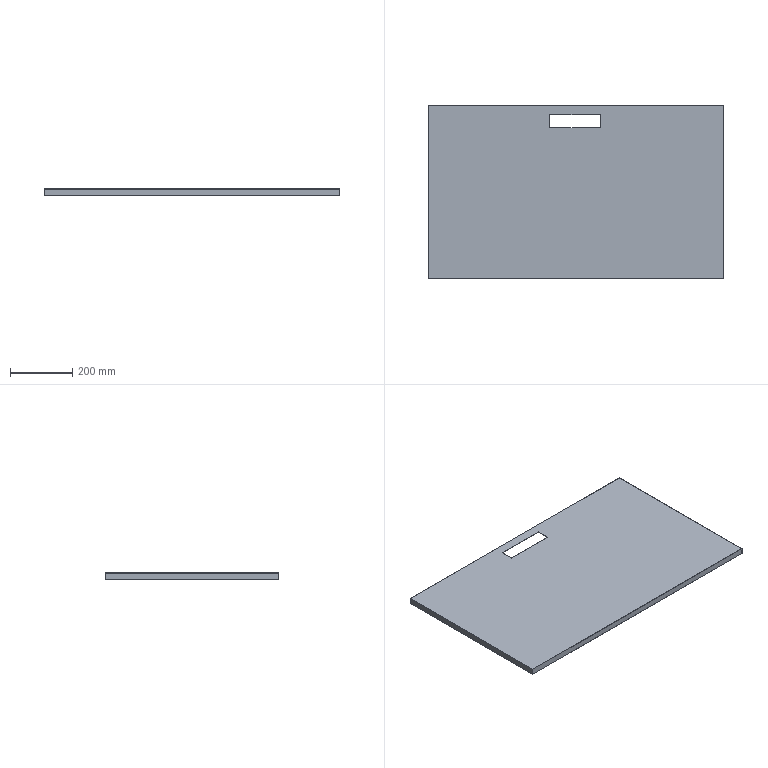Part | STEP file | PN_0019 | 1 solid | 15 faces | box 953 x 560 x 20 mm | volume 584212 mm3 | plane 15
STEP:
#1=CARTESIAN_POINT('',(0.,0.,0.));
#2=DIRECTION('',(0.,0.,1.));
#3=DIRECTION('',(1.,0.,0.));
#4=AXIS2_PLACEMENT_3D('',#1,#2,#3);
#5=CARTESIAN_POINT('',(0.,560.,0.));
#6=VERTEX_POINT('',#5);
#7=CARTESIAN_POINT('',(0.,0.,0.));
#8=VERTEX_POINT('',#7);
#9=CARTESIAN_POINT('',(0.,0.,0.));
#10=DIRECTION('',(0.,-1.,0.));
#11=VECTOR('',#10,1.);
#12=LINE('',#9,#11);
#13=CARTESIAN_POINT('',(0.,0.,0.));
#14=DIRECTION('',(0.,0.,-1.));
#15=DIRECTION('',(-1.,0.,0.));
#16=AXIS2_PLACEMENT_3D('',#13,#14,#15);
#17=PLANE('',#16);
#18=CARTESIAN_POINT('',(0.,0.));
#19=DIRECTION('',(0.,-1.));
#20=VECTOR('',#19,1.);
#21=LINE('',#18,#20);
#22=(GEOMETRIC_REPRESENTATION_CONTEXT(2)PARAMETRIC_REPRESENTATION_CONTEXT()REPRESENTATION_CONTEXT('',''));
#23=DEFINITIONAL_REPRESENTATION('',(#21),#22);
#24=PCURVE('',#17,#23);
#25=CARTESIAN_POINT('',(0.,0.,20.));
#26=DIRECTION('',(1.,0.,0.));
#27=DIRECTION('',(0.,0.,-1.));
#28=AXIS2_PLACEMENT_3D('',#25,#26,#27);
#29=PLANE('',#28);
#30=CARTESIAN_POINT('',(20.,0.));
#31=DIRECTION('',(0.,-1.));
#32=VECTOR('',#31,1.);
#33=LINE('',#30,#32);
#34=(GEOMETRIC_REPRESENTATION_CONTEXT(2)PARAMETRIC_REPRESENTATION_CONTEXT()REPRESENTATION_CONTEXT('',''));
#35=DEFINITIONAL_REPRESENTATION('',(#33),#34);
#36=PCURVE('',#29,#35);
#37=SURFACE_CURVE('',#12,(#24,#36),.PCURVE_S1.);
#38=EDGE_CURVE('',#6,#8,#37,.T.);
#39=ORIENTED_EDGE('',*,*,#38,.F.);
#40=CARTESIAN_POINT('',(953.,560.,0.));
#41=VERTEX_POINT('',#40);
#42=CARTESIAN_POINT('',(0.,560.,0.));
#43=DIRECTION('',(-1.,0.,0.));
#44=VECTOR('',#43,1.);
#45=LINE('',#42,#44);
#46=CARTESIAN_POINT('',(0.,560.));
#47=DIRECTION('',(1.,0.));
#48=VECTOR('',#47,1.);
#49=LINE('',#46,#48);
#50=(GEOMETRIC_REPRESENTATION_CONTEXT(2)PARAMETRIC_REPRESENTATION_CONTEXT()REPRESENTATION_CONTEXT('',''));
#51=DEFINITIONAL_REPRESENTATION('',(#49),#50);
#52=PCURVE('',#17,#51);
#53=CARTESIAN_POINT('',(0.,560.,20.));
#54=DIRECTION('',(0.,-1.,0.));
#55=DIRECTION('',(0.,0.,-1.));
#56=AXIS2_PLACEMENT_3D('',#53,#54,#55);
#57=PLANE('',#56);
#58=CARTESIAN_POINT('',(20.,0.));
#59=DIRECTION('',(0.,-1.));
#60=VECTOR('',#59,1.);
#61=LINE('',#58,#60);
#62=(GEOMETRIC_REPRESENTATION_CONTEXT(2)PARAMETRIC_REPRESENTATION_CONTEXT()REPRESENTATION_CONTEXT('',''));
#63=DEFINITIONAL_REPRESENTATION('',(#61),#62);
#64=PCURVE('',#57,#63);
#65=SURFACE_CURVE('',#45,(#52,#64),.PCURVE_S1.);
#66=EDGE_CURVE('',#41,#6,#65,.T.);
#67=ORIENTED_EDGE('',*,*,#66,.F.);
#68=CARTESIAN_POINT('',(953.,0.,0.));
#69=VERTEX_POINT('',#68);
#70=CARTESIAN_POINT('',(953.,0.,0.));
#71=DIRECTION('',(0.,1.,0.));
#72=VECTOR('',#71,1.);
#73=LINE('',#70,#72);
#74=CARTESIAN_POINT('',(-953.,0.));
#75=DIRECTION('',(0.,1.));
#76=VECTOR('',#75,1.);
#77=LINE('',#74,#76);
#78=(GEOMETRIC_REPRESENTATION_CONTEXT(2)PARAMETRIC_REPRESENTATION_CONTEXT()REPRESENTATION_CONTEXT('',''));
#79=DEFINITIONAL_REPRESENTATION('',(#77),#78);
#80=PCURVE('',#17,#79);
#81=CARTESIAN_POINT('',(953.,0.,20.));
#82=DIRECTION('',(-1.,0.,0.));
#83=DIRECTION('',(0.,0.,1.));
#84=AXIS2_PLACEMENT_3D('',#81,#82,#83);
#85=PLANE('',#84);
#86=CARTESIAN_POINT('',(-20.,0.));
#87=DIRECTION('',(0.,1.));
#88=VECTOR('',#87,1.);
#89=LINE('',#86,#88);
#90=(GEOMETRIC_REPRESENTATION_CONTEXT(2)PARAMETRIC_REPRESENTATION_CONTEXT()REPRESENTATION_CONTEXT('',''));
#91=DEFINITIONAL_REPRESENTATION('',(#89),#90);
#92=PCURVE('',#85,#91);
#93=SURFACE_CURVE('',#73,(#80,#92),.PCURVE_S1.);
#94=EDGE_CURVE('',#69,#41,#93,.T.);
#95=ORIENTED_EDGE('',*,*,#94,.F.);
#96=CARTESIAN_POINT('',(0.,0.,0.));
#97=DIRECTION('',(1.,0.,0.));
#98=VECTOR('',#97,1.);
#99=LINE('',#96,#98);
#100=CARTESIAN_POINT('',(0.,0.));
#101=DIRECTION('',(-1.,0.));
#102=VECTOR('',#101,1.);
#103=LINE('',#100,#102);
#104=(GEOMETRIC_REPRESENTATION_CONTEXT(2)PARAMETRIC_REPRESENTATION_CONTEXT()REPRESENTATION_CONTEXT('',''));
#105=DEFINITIONAL_REPRESENTATION('',(#103),#104);
#106=PCURVE('',#17,#105);
#107=CARTESIAN_POINT('',(0.,0.,20.));
#108=DIRECTION('',(0.,1.,0.));
#109=DIRECTION('',(0.,0.,1.));
#110=AXIS2_PLACEMENT_3D('',#107,#108,#109);
#111=PLANE('',#110);
#112=CARTESIAN_POINT('',(-20.,0.));
#113=DIRECTION('',(0.,1.));
#114=VECTOR('',#113,1.);
#115=LINE('',#112,#114);
#116=(GEOMETRIC_REPRESENTATION_CONTEXT(2)PARAMETRIC_REPRESENTATION_CONTEXT()REPRESENTATION_CONTEXT('',''));
#117=DEFINITIONAL_REPRESENTATION('',(#115),#116);
#118=PCURVE('',#111,#117);
#119=SURFACE_CURVE('',#99,(#106,#118),.PCURVE_S1.);
#120=EDGE_CURVE('',#8,#69,#119,.T.);
#121=ORIENTED_EDGE('',*,*,#120,.F.);
#122=EDGE_LOOP('',(#39,#67,#95,#121));
#123=FACE_BOUND('',#122,.T.);
#124=CARTESIAN_POINT('',(952.,559.,0.));
#125=VERTEX_POINT('',#124);
#126=CARTESIAN_POINT('',(1.,559.,0.));
#127=VERTEX_POINT('',#126);
#128=CARTESIAN_POINT('',(0.,559.,0.));
#129=DIRECTION('',(-1.,0.,0.));
#130=VECTOR('',#129,1.);
#131=LINE('',#128,#130);
#132=CARTESIAN_POINT('',(0.,559.));
#133=DIRECTION('',(1.,0.));
#134=VECTOR('',#133,1.);
#135=LINE('',#132,#134);
#136=(GEOMETRIC_REPRESENTATION_CONTEXT(2)PARAMETRIC_REPRESENTATION_CONTEXT()REPRESENTATION_CONTEXT('',''));
#137=DEFINITIONAL_REPRESENTATION('',(#135),#136);
#138=PCURVE('',#17,#137);
#139=CARTESIAN_POINT('',(0.,559.,20.));
#140=DIRECTION('',(0.,-1.,0.));
#141=DIRECTION('',(0.,0.,-1.));
#142=AXIS2_PLACEMENT_3D('',#139,#140,#141);
#143=PLANE('',#142);
#144=CARTESIAN_POINT('',(20.,0.));
#145=DIRECTION('',(0.,-1.));
#146=VECTOR('',#145,1.);
#147=LINE('',#144,#146);
#148=(GEOMETRIC_REPRESENTATION_CONTEXT(2)PARAMETRIC_REPRESENTATION_CONTEXT()REPRESENTATION_CONTEXT('',''));
#149=DEFINITIONAL_REPRESENTATION('',(#147),#148);
#150=PCURVE('',#143,#149);
#151=SURFACE_CURVE('',#131,(#138,#150),.PCURVE_S1.);
#152=EDGE_CURVE('',#125,#127,#151,.T.);
#153=ORIENTED_EDGE('',*,*,#152,.T.);
#154=CARTESIAN_POINT('',(1.,1.,0.));
#155=VERTEX_POINT('',#154);
#156=CARTESIAN_POINT('',(1.,0.,0.));
#157=DIRECTION('',(0.,-1.,0.));
#158=VECTOR('',#157,1.);
#159=LINE('',#156,#158);
#160=CARTESIAN_POINT('',(-1.,0.));
#161=DIRECTION('',(0.,-1.));
#162=VECTOR('',#161,1.);
#163=LINE('',#160,#162);
#164=(GEOMETRIC_REPRESENTATION_CONTEXT(2)PARAMETRIC_REPRESENTATION_CONTEXT()REPRESENTATION_CONTEXT('',''));
#165=DEFINITIONAL_REPRESENTATION('',(#163),#164);
#166=PCURVE('',#17,#165);
#167=CARTESIAN_POINT('',(1.,0.,20.));
#168=DIRECTION('',(1.,0.,0.));
#169=DIRECTION('',(0.,0.,-1.));
#170=AXIS2_PLACEMENT_3D('',#167,#168,#169);
#171=PLANE('',#170);
#172=CARTESIAN_POINT('',(20.,0.));
#173=DIRECTION('',(0.,-1.));
#174=VECTOR('',#173,1.);
#175=LINE('',#172,#174);
#176=(GEOMETRIC_REPRESENTATION_CONTEXT(2)PARAMETRIC_REPRESENTATION_CONTEXT()REPRESENTATION_CONTEXT('',''));
#177=DEFINITIONAL_REPRESENTATION('',(#175),#176);
#178=PCURVE('',#171,#177);
#179=SURFACE_CURVE('',#159,(#166,#178),.PCURVE_S1.);
#180=EDGE_CURVE('',#127,#155,#179,.T.);
#181=ORIENTED_EDGE('',*,*,#180,.T.);
#182=CARTESIAN_POINT('',(952.,1.,0.));
#183=VERTEX_POINT('',#182);
#184=CARTESIAN_POINT('',(0.,1.,0.));
#185=DIRECTION('',(1.,0.,0.));
#186=VECTOR('',#185,1.);
#187=LINE('',#184,#186);
#188=CARTESIAN_POINT('',(0.,1.));
#189=DIRECTION('',(-1.,0.));
#190=VECTOR('',#189,1.);
#191=LINE('',#188,#190);
#192=(GEOMETRIC_REPRESENTATION_CONTEXT(2)PARAMETRIC_REPRESENTATION_CONTEXT()REPRESENTATION_CONTEXT('',''));
#193=DEFINITIONAL_REPRESENTATION('',(#191),#192);
#194=PCURVE('',#17,#193);
#195=CARTESIAN_POINT('',(0.,1.,20.));
#196=DIRECTION('',(0.,1.,0.));
#197=DIRECTION('',(0.,0.,1.));
#198=AXIS2_PLACEMENT_3D('',#195,#196,#197);
#199=PLANE('',#198);
#200=CARTESIAN_POINT('',(-20.,0.));
#201=DIRECTION('',(0.,1.));
#202=VECTOR('',#201,1.);
#203=LINE('',#200,#202);
#204=(GEOMETRIC_REPRESENTATION_CONTEXT(2)PARAMETRIC_REPRESENTATION_CONTEXT()REPRESENTATION_CONTEXT('',''));
#205=DEFINITIONAL_REPRESENTATION('',(#203),#204);
#206=PCURVE('',#199,#205);
#207=SURFACE_CURVE('',#187,(#194,#206),.PCURVE_S1.);
#208=EDGE_CURVE('',#155,#183,#207,.T.);
#209=ORIENTED_EDGE('',*,*,#208,.T.);
#210=CARTESIAN_POINT('',(952.,0.,0.));
#211=DIRECTION('',(0.,1.,0.));
#212=VECTOR('',#211,1.);
#213=LINE('',#210,#212);
#214=CARTESIAN_POINT('',(-952.,0.));
#215=DIRECTION('',(0.,1.));
#216=VECTOR('',#215,1.);
#217=LINE('',#214,#216);
#218=(GEOMETRIC_REPRESENTATION_CONTEXT(2)PARAMETRIC_REPRESENTATION_CONTEXT()REPRESENTATION_CONTEXT('',''));
#219=DEFINITIONAL_REPRESENTATION('',(#217),#218);
#220=PCURVE('',#17,#219);
#221=CARTESIAN_POINT('',(952.,0.,20.));
#222=DIRECTION('',(-1.,0.,0.));
#223=DIRECTION('',(0.,0.,1.));
#224=AXIS2_PLACEMENT_3D('',#221,#222,#223);
#225=PLANE('',#224);
#226=CARTESIAN_POINT('',(-20.,0.));
#227=DIRECTION('',(0.,1.));
#228=VECTOR('',#227,1.);
#229=LINE('',#226,#228);
#230=(GEOMETRIC_REPRESENTATION_CONTEXT(2)PARAMETRIC_REPRESENTATION_CONTEXT()REPRESENTATION_CONTEXT('',''));
#231=DEFINITIONAL_REPRESENTATION('',(#229),#230);
#232=PCURVE('',#225,#231);
#233=SURFACE_CURVE('',#213,(#220,#232),.PCURVE_S1.);
#234=EDGE_CURVE('',#183,#125,#233,.T.);
#235=ORIENTED_EDGE('',*,*,#234,.T.);
#236=EDGE_LOOP('',(#153,#181,#209,#235));
#237=FACE_BOUND('',#236,.T.);
#238=ADVANCED_FACE('',(#123,#237),#17,.T.);
#239=ORIENTED_EDGE('',*,*,#38,.T.);
#240=CARTESIAN_POINT('',(0.,0.,20.));
#241=VERTEX_POINT('',#240);
#242=CARTESIAN_POINT('',(0.,0.,20.));
#243=DIRECTION('',(0.,0.,-1.));
#244=VECTOR('',#243,1.);
#245=LINE('',#242,#244);
#246=CARTESIAN_POINT('',(0.,0.));
#247=DIRECTION('',(1.,0.));
#248=VECTOR('',#247,1.);
#249=LINE('',#246,#248);
#250=(GEOMETRIC_REPRESENTATION_CONTEXT(2)PARAMETRIC_REPRESENTATION_CONTEXT()REPRESENTATION_CONTEXT('',''));
#251=DEFINITIONAL_REPRESENTATION('',(#249),#250);
#252=PCURVE('',#29,#251);
#253=CARTESIAN_POINT('',(0.,0.));
#254=DIRECTION('',(-1.,0.));
#255=VECTOR('',#254,1.);
#256=LINE('',#253,#255);
#257=(GEOMETRIC_REPRESENTATION_CONTEXT(2)PARAMETRIC_REPRESENTATION_CONTEXT()REPRESENTATION_CONTEXT('',''));
#258=DEFINITIONAL_REPRESENTATION('',(#256),#257);
#259=PCURVE('',#111,#258);
#260=SURFACE_CURVE('',#245,(#252,#259),.PCURVE_S1.);
#261=EDGE_CURVE('',#241,#8,#260,.T.);
#262=ORIENTED_EDGE('',*,*,#261,.F.);
#263=CARTESIAN_POINT('',(0.,560.,20.));
#264=VERTEX_POINT('',#263);
#265=CARTESIAN_POINT('',(0.,0.,20.));
#266=DIRECTION('',(0.,-1.,0.));
#267=VECTOR('',#266,1.);
#268=LINE('',#265,#267);
#269=CARTESIAN_POINT('',(0.,0.));
#270=DIRECTION('',(0.,-1.));
#271=VECTOR('',#270,1.);
#272=LINE('',#269,#271);
#273=(GEOMETRIC_REPRESENTATION_CONTEXT(2)PARAMETRIC_REPRESENTATION_CONTEXT()REPRESENTATION_CONTEXT('',''));
#274=DEFINITIONAL_REPRESENTATION('',(#272),#273);
#275=PCURVE('',#29,#274);
#276=CARTESIAN_POINT('',(0.,0.,20.));
#277=DIRECTION('',(0.,0.,-1.));
#278=DIRECTION('',(-1.,0.,0.));
#279=AXIS2_PLACEMENT_3D('',#276,#277,#278);
#280=PLANE('',#279);
#281=CARTESIAN_POINT('',(0.,0.));
#282=DIRECTION('',(0.,-1.));
#283=VECTOR('',#282,1.);
#284=LINE('',#281,#283);
#285=(GEOMETRIC_REPRESENTATION_CONTEXT(2)PARAMETRIC_REPRESENTATION_CONTEXT()REPRESENTATION_CONTEXT('',''));
#286=DEFINITIONAL_REPRESENTATION('',(#284),#285);
#287=PCURVE('',#280,#286);
#288=SURFACE_CURVE('',#268,(#275,#287),.PCURVE_S1.);
#289=EDGE_CURVE('',#264,#241,#288,.T.);
#290=ORIENTED_EDGE('',*,*,#289,.F.);
#291=CARTESIAN_POINT('',(0.,560.,20.));
#292=DIRECTION('',(0.,0.,-1.));
#293=VECTOR('',#292,1.);
#294=LINE('',#291,#293);
#295=CARTESIAN_POINT('',(0.,560.));
#296=DIRECTION('',(1.,0.));
#297=VECTOR('',#296,1.);
#298=LINE('',#295,#297);
#299=(GEOMETRIC_REPRESENTATION_CONTEXT(2)PARAMETRIC_REPRESENTATION_CONTEXT()REPRESENTATION_CONTEXT('',''));
#300=DEFINITIONAL_REPRESENTATION('',(#298),#299);
#301=PCURVE('',#29,#300);
#302=CARTESIAN_POINT('',(0.,0.));
#303=DIRECTION('',(1.,0.));
#304=VECTOR('',#303,1.);
#305=LINE('',#302,#304);
#306=(GEOMETRIC_REPRESENTATION_CONTEXT(2)PARAMETRIC_REPRESENTATION_CONTEXT()REPRESENTATION_CONTEXT('',''));
#307=DEFINITIONAL_REPRESENTATION('',(#305),#306);
#308=PCURVE('',#57,#307);
#309=SURFACE_CURVE('',#294,(#301,#308),.PCURVE_S1.);
#310=EDGE_CURVE('',#264,#6,#309,.T.);
#311=ORIENTED_EDGE('',*,*,#310,.T.);
#312=EDGE_LOOP('',(#239,#262,#290,#311));
#313=FACE_BOUND('',#312,.T.);
#314=ADVANCED_FACE('',(#313),#29,.F.);
#315=ORIENTED_EDGE('',*,*,#120,.T.);
#316=CARTESIAN_POINT('',(953.,0.,20.));
#317=VERTEX_POINT('',#316);
#318=CARTESIAN_POINT('',(953.,0.,20.));
#319=DIRECTION('',(0.,0.,-1.));
#320=VECTOR('',#319,1.);
#321=LINE('',#318,#320);
#322=CARTESIAN_POINT('',(0.,953.));
#323=DIRECTION('',(-1.,0.));
#324=VECTOR('',#323,1.);
#325=LINE('',#322,#324);
#326=(GEOMETRIC_REPRESENTATION_CONTEXT(2)PARAMETRIC_REPRESENTATION_CONTEXT()REPRESENTATION_CONTEXT('',''));
#327=DEFINITIONAL_REPRESENTATION('',(#325),#326);
#328=PCURVE('',#111,#327);
#329=CARTESIAN_POINT('',(0.,0.));
#330=DIRECTION('',(-1.,0.));
#331=VECTOR('',#330,1.);
#332=LINE('',#329,#331);
#333=(GEOMETRIC_REPRESENTATION_CONTEXT(2)PARAMETRIC_REPRESENTATION_CONTEXT()REPRESENTATION_CONTEXT('',''));
#334=DEFINITIONAL_REPRESENTATION('',(#332),#333);
#335=PCURVE('',#85,#334);
#336=SURFACE_CURVE('',#321,(#328,#335),.PCURVE_S1.);
#337=EDGE_CURVE('',#317,#69,#336,.T.);
#338=ORIENTED_EDGE('',*,*,#337,.F.);
#339=CARTESIAN_POINT('',(0.,0.,20.));
#340=DIRECTION('',(1.,0.,0.));
#341=VECTOR('',#340,1.);
#342=LINE('',#339,#341);
#343=CARTESIAN_POINT('',(0.,0.));
#344=DIRECTION('',(0.,1.));
#345=VECTOR('',#344,1.);
#346=LINE('',#343,#345);
#347=(GEOMETRIC_REPRESENTATION_CONTEXT(2)PARAMETRIC_REPRESENTATION_CONTEXT()REPRESENTATION_CONTEXT('',''));
#348=DEFINITIONAL_REPRESENTATION('',(#346),#347);
#349=PCURVE('',#111,#348);
#350=CARTESIAN_POINT('',(0.,0.));
#351=DIRECTION('',(-1.,0.));
#352=VECTOR('',#351,1.);
#353=LINE('',#350,#352);
#354=(GEOMETRIC_REPRESENTATION_CONTEXT(2)PARAMETRIC_REPRESENTATION_CONTEXT()REPRESENTATION_CONTEXT('',''));
#355=DEFINITIONAL_REPRESENTATION('',(#353),#354);
#356=PCURVE('',#280,#355);
#357=SURFACE_CURVE('',#342,(#349,#356),.PCURVE_S1.);
#358=EDGE_CURVE('',#241,#317,#357,.T.);
#359=ORIENTED_EDGE('',*,*,#358,.F.);
#360=ORIENTED_EDGE('',*,*,#261,.T.);
#361=EDGE_LOOP('',(#315,#338,#359,#360));
#362=FACE_BOUND('',#361,.T.);
#363=ADVANCED_FACE('',(#362),#111,.F.);
#364=ORIENTED_EDGE('',*,*,#94,.T.);
#365=CARTESIAN_POINT('',(953.,560.,20.));
#366=VERTEX_POINT('',#365);
#367=CARTESIAN_POINT('',(953.,560.,20.));
#368=DIRECTION('',(0.,0.,-1.));
#369=VECTOR('',#368,1.);
#370=LINE('',#367,#369);
#371=CARTESIAN_POINT('',(0.,560.));
#372=DIRECTION('',(-1.,0.));
#373=VECTOR('',#372,1.);
#374=LINE('',#371,#373);
#375=(GEOMETRIC_REPRESENTATION_CONTEXT(2)PARAMETRIC_REPRESENTATION_CONTEXT()REPRESENTATION_CONTEXT('',''));
#376=DEFINITIONAL_REPRESENTATION('',(#374),#375);
#377=PCURVE('',#85,#376);
#378=CARTESIAN_POINT('',(0.,953.));
#379=DIRECTION('',(1.,0.));
#380=VECTOR('',#379,1.);
#381=LINE('',#378,#380);
#382=(GEOMETRIC_REPRESENTATION_CONTEXT(2)PARAMETRIC_REPRESENTATION_CONTEXT()REPRESENTATION_CONTEXT('',''));
#383=DEFINITIONAL_REPRESENTATION('',(#381),#382);
#384=PCURVE('',#57,#383);
#385=SURFACE_CURVE('',#370,(#377,#384),.PCURVE_S1.);
#386=EDGE_CURVE('',#366,#41,#385,.T.);
#387=ORIENTED_EDGE('',*,*,#386,.F.);
#388=CARTESIAN_POINT('',(953.,0.,20.));
#389=DIRECTION('',(0.,1.,0.));
#390=VECTOR('',#389,1.);
#391=LINE('',#388,#390);
#392=CARTESIAN_POINT('',(0.,0.));
#393=DIRECTION('',(0.,1.));
#394=VECTOR('',#393,1.);
#395=LINE('',#392,#394);
#396=(GEOMETRIC_REPRESENTATION_CONTEXT(2)PARAMETRIC_REPRESENTATION_CONTEXT()REPRESENTATION_CONTEXT('',''));
#397=DEFINITIONAL_REPRESENTATION('',(#395),#396);
#398=PCURVE('',#85,#397);
#399=CARTESIAN_POINT('',(-953.,0.));
#400=DIRECTION('',(0.,1.));
#401=VECTOR('',#400,1.);
#402=LINE('',#399,#401);
#403=(GEOMETRIC_REPRESENTATION_CONTEXT(2)PARAMETRIC_REPRESENTATION_CONTEXT()REPRESENTATION_CONTEXT('',''));
#404=DEFINITIONAL_REPRESENTATION('',(#402),#403);
#405=PCURVE('',#280,#404);
#406=SURFACE_CURVE('',#391,(#398,#405),.PCURVE_S1.);
#407=EDGE_CURVE('',#317,#366,#406,.T.);
#408=ORIENTED_EDGE('',*,*,#407,.F.);
#409=ORIENTED_EDGE('',*,*,#337,.T.);
#410=EDGE_LOOP('',(#364,#387,#408,#409));
#411=FACE_BOUND('',#410,.T.);
#412=ADVANCED_FACE('',(#411),#85,.F.);
#413=ORIENTED_EDGE('',*,*,#66,.T.);
#414=ORIENTED_EDGE('',*,*,#310,.F.);
#415=CARTESIAN_POINT('',(0.,560.,20.));
#416=DIRECTION('',(-1.,0.,0.));
#417=VECTOR('',#416,1.);
#418=LINE('',#415,#417);
#419=CARTESIAN_POINT('',(0.,0.));
#420=DIRECTION('',(0.,-1.));
#421=VECTOR('',#420,1.);
#422=LINE('',#419,#421);
#423=(GEOMETRIC_REPRESENTATION_CONTEXT(2)PARAMETRIC_REPRESENTATION_CONTEXT()REPRESENTATION_CONTEXT('',''));
#424=DEFINITIONAL_REPRESENTATION('',(#422),#423);
#425=PCURVE('',#57,#424);
#426=CARTESIAN_POINT('',(0.,560.));
#427=DIRECTION('',(1.,0.));
#428=VECTOR('',#427,1.);
#429=LINE('',#426,#428);
#430=(GEOMETRIC_REPRESENTATION_CONTEXT(2)PARAMETRIC_REPRESENTATION_CONTEXT()REPRESENTATION_CONTEXT('',''));
#431=DEFINITIONAL_REPRESENTATION('',(#429),#430);
#432=PCURVE('',#280,#431);
#433=SURFACE_CURVE('',#418,(#425,#432),.PCURVE_S1.);
#434=EDGE_CURVE('',#366,#264,#433,.T.);
#435=ORIENTED_EDGE('',*,*,#434,.F.);
#436=ORIENTED_EDGE('',*,*,#386,.T.);
#437=EDGE_LOOP('',(#413,#414,#435,#436));
#438=FACE_BOUND('',#437,.T.);
#439=ADVANCED_FACE('',(#438),#57,.F.);
#440=CARTESIAN_POINT('',(555.662,529.213,20.));
#441=VERTEX_POINT('',#440);
#442=CARTESIAN_POINT('',(391.367,529.213,20.));
#443=VERTEX_POINT('',#442);
#444=CARTESIAN_POINT('',(555.662,529.213,20.));
#445=DIRECTION('',(-1.,0.,0.));
#446=VECTOR('',#445,1.);
#447=LINE('',#444,#446);
#448=CARTESIAN_POINT('',(-555.662,529.213));
#449=DIRECTION('',(1.,0.));
#450=VECTOR('',#449,1.);
#451=LINE('',#448,#450);
#452=(GEOMETRIC_REPRESENTATION_CONTEXT(2)PARAMETRIC_REPRESENTATION_CONTEXT()REPRESENTATION_CONTEXT('',''));
#453=DEFINITIONAL_REPRESENTATION('',(#451),#452);
#454=PCURVE('',#280,#453);
#455=CARTESIAN_POINT('',(555.662,529.213,10.));
#456=DIRECTION('',(0.,1.,0.));
#457=DIRECTION('',(0.,0.,1.));
#458=AXIS2_PLACEMENT_3D('',#455,#456,#457);
#459=PLANE('',#458);
#460=CARTESIAN_POINT('',(10.,0.));
#461=DIRECTION('',(0.,-1.));
#462=VECTOR('',#461,1.);
#463=LINE('',#460,#462);
#464=(GEOMETRIC_REPRESENTATION_CONTEXT(2)PARAMETRIC_REPRESENTATION_CONTEXT()REPRESENTATION_CONTEXT('',''));
#465=DEFINITIONAL_REPRESENTATION('',(#463),#464);
#466=PCURVE('',#459,#465);
#467=SURFACE_CURVE('',#447,(#454,#466),.PCURVE_S1.);
#468=EDGE_CURVE('',#441,#443,#467,.T.);
#469=ORIENTED_EDGE('',*,*,#468,.F.);
#470=CARTESIAN_POINT('',(555.662,487.3,20.));
#471=VERTEX_POINT('',#470);
#472=CARTESIAN_POINT('',(555.662,529.213,20.));
#473=DIRECTION('',(0.,1.,0.));
#474=VECTOR('',#473,1.);
#475=LINE('',#472,#474);
#476=CARTESIAN_POINT('',(-555.662,529.213));
#477=DIRECTION('',(0.,1.));
#478=VECTOR('',#477,1.);
#479=LINE('',#476,#478);
#480=(GEOMETRIC_REPRESENTATION_CONTEXT(2)PARAMETRIC_REPRESENTATION_CONTEXT()REPRESENTATION_CONTEXT('',''));
#481=DEFINITIONAL_REPRESENTATION('',(#479),#480);
#482=PCURVE('',#280,#481);
#483=CARTESIAN_POINT('',(555.662,529.213,10.));
#484=DIRECTION('',(1.,0.,0.));
#485=DIRECTION('',(0.,0.,-1.));
#486=AXIS2_PLACEMENT_3D('',#483,#484,#485);
#487=PLANE('',#486);
#488=CARTESIAN_POINT('',(-10.,0.));
#489=DIRECTION('',(0.,1.));
#490=VECTOR('',#489,1.);
#491=LINE('',#488,#490);
#492=(GEOMETRIC_REPRESENTATION_CONTEXT(2)PARAMETRIC_REPRESENTATION_CONTEXT()REPRESENTATION_CONTEXT('',''));
#493=DEFINITIONAL_REPRESENTATION('',(#491),#492);
#494=PCURVE('',#487,#493);
#495=SURFACE_CURVE('',#475,(#482,#494),.PCURVE_S1.);
#496=EDGE_CURVE('',#471,#441,#495,.T.);
#497=ORIENTED_EDGE('',*,*,#496,.F.);
#498=CARTESIAN_POINT('',(391.367,487.3,20.));
#499=VERTEX_POINT('',#498);
#500=CARTESIAN_POINT('',(555.662,487.3,20.));
#501=DIRECTION('',(1.,0.,0.));
#502=VECTOR('',#501,1.);
#503=LINE('',#500,#502);
#504=CARTESIAN_POINT('',(-555.662,487.3));
#505=DIRECTION('',(-1.,0.));
#506=VECTOR('',#505,1.);
#507=LINE('',#504,#506);
#508=(GEOMETRIC_REPRESENTATION_CONTEXT(2)PARAMETRIC_REPRESENTATION_CONTEXT()REPRESENTATION_CONTEXT('',''));
#509=DEFINITIONAL_REPRESENTATION('',(#507),#508);
#510=PCURVE('',#280,#509);
#511=CARTESIAN_POINT('',(555.662,487.3,10.));
#512=DIRECTION('',(0.,-1.,0.));
#513=DIRECTION('',(0.,0.,-1.));
#514=AXIS2_PLACEMENT_3D('',#511,#512,#513);
#515=PLANE('',#514);
#516=CARTESIAN_POINT('',(-10.,0.));
#517=DIRECTION('',(0.,1.));
#518=VECTOR('',#517,1.);
#519=LINE('',#516,#518);
#520=(GEOMETRIC_REPRESENTATION_CONTEXT(2)PARAMETRIC_REPRESENTATION_CONTEXT()REPRESENTATION_CONTEXT('',''));
#521=DEFINITIONAL_REPRESENTATION('',(#519),#520);
#522=PCURVE('',#515,#521);
#523=SURFACE_CURVE('',#503,(#510,#522),.PCURVE_S1.);
#524=EDGE_CURVE('',#499,#471,#523,.T.);
#525=ORIENTED_EDGE('',*,*,#524,.F.);
#526=CARTESIAN_POINT('',(391.367,529.213,20.));
#527=DIRECTION('',(0.,-1.,0.));
#528=VECTOR('',#527,1.);
#529=LINE('',#526,#528);
#530=CARTESIAN_POINT('',(-391.367,529.213));
#531=DIRECTION('',(0.,-1.));
#532=VECTOR('',#531,1.);
#533=LINE('',#530,#532);
#534=(GEOMETRIC_REPRESENTATION_CONTEXT(2)PARAMETRIC_REPRESENTATION_CONTEXT()REPRESENTATION_CONTEXT('',''));
#535=DEFINITIONAL_REPRESENTATION('',(#533),#534);
#536=PCURVE('',#280,#535);
#537=CARTESIAN_POINT('',(391.367,529.213,10.));
#538=DIRECTION('',(-1.,0.,0.));
#539=DIRECTION('',(0.,0.,1.));
#540=AXIS2_PLACEMENT_3D('',#537,#538,#539);
#541=PLANE('',#540);
#542=CARTESIAN_POINT('',(10.,0.));
#543=DIRECTION('',(0.,-1.));
#544=VECTOR('',#543,1.);
#545=LINE('',#542,#544);
#546=(GEOMETRIC_REPRESENTATION_CONTEXT(2)PARAMETRIC_REPRESENTATION_CONTEXT()REPRESENTATION_CONTEXT('',''));
#547=DEFINITIONAL_REPRESENTATION('',(#545),#546);
#548=PCURVE('',#541,#547);
#549=SURFACE_CURVE('',#529,(#536,#548),.PCURVE_S1.);
#550=EDGE_CURVE('',#443,#499,#549,.T.);
#551=ORIENTED_EDGE('',*,*,#550,.F.);
#552=EDGE_LOOP('',(#469,#497,#525,#551));
#553=FACE_BOUND('',#552,.T.);
#554=ORIENTED_EDGE('',*,*,#289,.T.);
#555=ORIENTED_EDGE('',*,*,#358,.T.);
#556=ORIENTED_EDGE('',*,*,#407,.T.);
#557=ORIENTED_EDGE('',*,*,#434,.T.);
#558=EDGE_LOOP('',(#554,#555,#556,#557));
#559=FACE_BOUND('',#558,.T.);
#560=ADVANCED_FACE('',(#553,#559),#280,.F.);
#561=ORIENTED_EDGE('',*,*,#180,.F.);
#562=CARTESIAN_POINT('',(1.,559.,19.));
#563=VERTEX_POINT('',#562);
#564=CARTESIAN_POINT('',(1.,559.,20.));
#565=DIRECTION('',(0.,0.,-1.));
#566=VECTOR('',#565,1.);
#567=LINE('',#564,#566);
#568=CARTESIAN_POINT('',(0.,559.));
#569=DIRECTION('',(1.,0.));
#570=VECTOR('',#569,1.);
#571=LINE('',#568,#570);
#572=(GEOMETRIC_REPRESENTATION_CONTEXT(2)PARAMETRIC_REPRESENTATION_CONTEXT()REPRESENTATION_CONTEXT('',''));
#573=DEFINITIONAL_REPRESENTATION('',(#571),#572);
#574=PCURVE('',#171,#573);
#575=CARTESIAN_POINT('',(0.,1.));
#576=DIRECTION('',(1.,0.));
#577=VECTOR('',#576,1.);
#578=LINE('',#575,#577);
#579=(GEOMETRIC_REPRESENTATION_CONTEXT(2)PARAMETRIC_REPRESENTATION_CONTEXT()REPRESENTATION_CONTEXT('',''));
#580=DEFINITIONAL_REPRESENTATION('',(#578),#579);
#581=PCURVE('',#143,#580);
#582=SURFACE_CURVE('',#567,(#574,#581),.PCURVE_S1.);
#583=EDGE_CURVE('',#563,#127,#582,.T.);
#584=ORIENTED_EDGE('',*,*,#583,.F.);
#585=CARTESIAN_POINT('',(1.,1.,19.));
#586=VERTEX_POINT('',#585);
#587=CARTESIAN_POINT('',(1.,0.,19.));
#588=DIRECTION('',(0.,-1.,0.));
#589=VECTOR('',#588,1.);
#590=LINE('',#587,#589);
#591=CARTESIAN_POINT('',(1.,0.));
#592=DIRECTION('',(0.,-1.));
#593=VECTOR('',#592,1.);
#594=LINE('',#591,#593);
#595=(GEOMETRIC_REPRESENTATION_CONTEXT(2)PARAMETRIC_REPRESENTATION_CONTEXT()REPRESENTATION_CONTEXT('',''));
#596=DEFINITIONAL_REPRESENTATION('',(#594),#595);
#597=PCURVE('',#171,#596);
#598=CARTESIAN_POINT('',(0.,0.,19.));
#599=DIRECTION('',(0.,0.,-1.));
#600=DIRECTION('',(-1.,0.,0.));
#601=AXIS2_PLACEMENT_3D('',#598,#599,#600);
#602=PLANE('',#601);
#603=CARTESIAN_POINT('',(-1.,0.));
#604=DIRECTION('',(0.,-1.));
#605=VECTOR('',#604,1.);
#606=LINE('',#603,#605);
#607=(GEOMETRIC_REPRESENTATION_CONTEXT(2)PARAMETRIC_REPRESENTATION_CONTEXT()REPRESENTATION_CONTEXT('',''));
#608=DEFINITIONAL_REPRESENTATION('',(#606),#607);
#609=PCURVE('',#602,#608);
#610=SURFACE_CURVE('',#590,(#597,#609),.PCURVE_S1.);
#611=EDGE_CURVE('',#563,#586,#610,.T.);
#612=ORIENTED_EDGE('',*,*,#611,.T.);
#613=CARTESIAN_POINT('',(1.,1.,20.));
#614=DIRECTION('',(0.,0.,-1.));
#615=VECTOR('',#614,1.);
#616=LINE('',#613,#615);
#617=CARTESIAN_POINT('',(0.,1.));
#618=DIRECTION('',(1.,0.));
#619=VECTOR('',#618,1.);
#620=LINE('',#617,#619);
#621=(GEOMETRIC_REPRESENTATION_CONTEXT(2)PARAMETRIC_REPRESENTATION_CONTEXT()REPRESENTATION_CONTEXT('',''));
#622=DEFINITIONAL_REPRESENTATION('',(#620),#621);
#623=PCURVE('',#171,#622);
#624=CARTESIAN_POINT('',(0.,1.));
#625=DIRECTION('',(-1.,0.));
#626=VECTOR('',#625,1.);
#627=LINE('',#624,#626);
#628=(GEOMETRIC_REPRESENTATION_CONTEXT(2)PARAMETRIC_REPRESENTATION_CONTEXT()REPRESENTATION_CONTEXT('',''));
#629=DEFINITIONAL_REPRESENTATION('',(#627),#628);
#630=PCURVE('',#199,#629);
#631=SURFACE_CURVE('',#616,(#623,#630),.PCURVE_S1.);
#632=EDGE_CURVE('',#586,#155,#631,.T.);
#633=ORIENTED_EDGE('',*,*,#632,.T.);
#634=EDGE_LOOP('',(#561,#584,#612,#633));
#635=FACE_BOUND('',#634,.T.);
#636=ADVANCED_FACE('',(#635),#171,.T.);
#637=ORIENTED_EDGE('',*,*,#208,.F.);
#638=ORIENTED_EDGE('',*,*,#632,.F.);
#639=CARTESIAN_POINT('',(952.,1.,19.));
#640=VERTEX_POINT('',#639);
#641=CARTESIAN_POINT('',(0.,1.,19.));
#642=DIRECTION('',(1.,0.,0.));
#643=VECTOR('',#642,1.);
#644=LINE('',#641,#643);
#645=CARTESIAN_POINT('',(-1.,0.));
#646=DIRECTION('',(0.,1.));
#647=VECTOR('',#646,1.);
#648=LINE('',#645,#647);
#649=(GEOMETRIC_REPRESENTATION_CONTEXT(2)PARAMETRIC_REPRESENTATION_CONTEXT()REPRESENTATION_CONTEXT('',''));
#650=DEFINITIONAL_REPRESENTATION('',(#648),#649);
#651=PCURVE('',#199,#650);
#652=CARTESIAN_POINT('',(0.,1.));
#653=DIRECTION('',(-1.,0.));
#654=VECTOR('',#653,1.);
#655=LINE('',#652,#654);
#656=(GEOMETRIC_REPRESENTATION_CONTEXT(2)PARAMETRIC_REPRESENTATION_CONTEXT()REPRESENTATION_CONTEXT('',''));
#657=DEFINITIONAL_REPRESENTATION('',(#655),#656);
#658=PCURVE('',#602,#657);
#659=SURFACE_CURVE('',#644,(#651,#658),.PCURVE_S1.);
#660=EDGE_CURVE('',#586,#640,#659,.T.);
#661=ORIENTED_EDGE('',*,*,#660,.T.);
#662=CARTESIAN_POINT('',(952.,1.,20.));
#663=DIRECTION('',(0.,0.,-1.));
#664=VECTOR('',#663,1.);
#665=LINE('',#662,#664);
#666=CARTESIAN_POINT('',(0.,952.));
#667=DIRECTION('',(-1.,0.));
#668=VECTOR('',#667,1.);
#669=LINE('',#666,#668);
#670=(GEOMETRIC_REPRESENTATION_CONTEXT(2)PARAMETRIC_REPRESENTATION_CONTEXT()REPRESENTATION_CONTEXT('',''));
#671=DEFINITIONAL_REPRESENTATION('',(#669),#670);
#672=PCURVE('',#199,#671);
#673=CARTESIAN_POINT('',(0.,1.));
#674=DIRECTION('',(-1.,0.));
#675=VECTOR('',#674,1.);
#676=LINE('',#673,#675);
#677=(GEOMETRIC_REPRESENTATION_CONTEXT(2)PARAMETRIC_REPRESENTATION_CONTEXT()REPRESENTATION_CONTEXT('',''));
#678=DEFINITIONAL_REPRESENTATION('',(#676),#677);
#679=PCURVE('',#225,#678);
#680=SURFACE_CURVE('',#665,(#672,#679),.PCURVE_S1.);
#681=EDGE_CURVE('',#640,#183,#680,.T.);
#682=ORIENTED_EDGE('',*,*,#681,.T.);
#683=EDGE_LOOP('',(#637,#638,#661,#682));
#684=FACE_BOUND('',#683,.T.);
#685=ADVANCED_FACE('',(#684),#199,.T.);
#686=ORIENTED_EDGE('',*,*,#234,.F.);
#687=ORIENTED_EDGE('',*,*,#681,.F.);
#688=CARTESIAN_POINT('',(952.,559.,19.));
#689=VERTEX_POINT('',#688);
#690=CARTESIAN_POINT('',(952.,0.,19.));
#691=DIRECTION('',(0.,1.,0.));
#692=VECTOR('',#691,1.);
#693=LINE('',#690,#692);
#694=CARTESIAN_POINT('',(-1.,0.));
#695=DIRECTION('',(0.,1.));
#696=VECTOR('',#695,1.);
#697=LINE('',#694,#696);
#698=(GEOMETRIC_REPRESENTATION_CONTEXT(2)PARAMETRIC_REPRESENTATION_CONTEXT()REPRESENTATION_CONTEXT('',''));
#699=DEFINITIONAL_REPRESENTATION('',(#697),#698);
#700=PCURVE('',#225,#699);
#701=CARTESIAN_POINT('',(-952.,0.));
#702=DIRECTION('',(0.,1.));
#703=VECTOR('',#702,1.);
#704=LINE('',#701,#703);
#705=(GEOMETRIC_REPRESENTATION_CONTEXT(2)PARAMETRIC_REPRESENTATION_CONTEXT()REPRESENTATION_CONTEXT('',''));
#706=DEFINITIONAL_REPRESENTATION('',(#704),#705);
#707=PCURVE('',#602,#706);
#708=SURFACE_CURVE('',#693,(#700,#707),.PCURVE_S1.);
#709=EDGE_CURVE('',#640,#689,#708,.T.);
#710=ORIENTED_EDGE('',*,*,#709,.T.);
#711=CARTESIAN_POINT('',(952.,559.,20.));
#712=DIRECTION('',(0.,0.,-1.));
#713=VECTOR('',#712,1.);
#714=LINE('',#711,#713);
#715=CARTESIAN_POINT('',(0.,559.));
#716=DIRECTION('',(-1.,0.));
#717=VECTOR('',#716,1.);
#718=LINE('',#715,#717);
#719=(GEOMETRIC_REPRESENTATION_CONTEXT(2)PARAMETRIC_REPRESENTATION_CONTEXT()REPRESENTATION_CONTEXT('',''));
#720=DEFINITIONAL_REPRESENTATION('',(#718),#719);
#721=PCURVE('',#225,#720);
#722=CARTESIAN_POINT('',(0.,952.));
#723=DIRECTION('',(1.,0.));
#724=VECTOR('',#723,1.);
#725=LINE('',#722,#724);
#726=(GEOMETRIC_REPRESENTATION_CONTEXT(2)PARAMETRIC_REPRESENTATION_CONTEXT()REPRESENTATION_CONTEXT('',''));
#727=DEFINITIONAL_REPRESENTATION('',(#725),#726);
#728=PCURVE('',#143,#727);
#729=SURFACE_CURVE('',#714,(#721,#728),.PCURVE_S1.);
#730=EDGE_CURVE('',#689,#125,#729,.T.);
#731=ORIENTED_EDGE('',*,*,#730,.T.);
#732=EDGE_LOOP('',(#686,#687,#710,#731));
#733=FACE_BOUND('',#732,.T.);
#734=ADVANCED_FACE('',(#733),#225,.T.);
#735=ORIENTED_EDGE('',*,*,#152,.F.);
#736=ORIENTED_EDGE('',*,*,#730,.F.);
#737=CARTESIAN_POINT('',(0.,559.,19.));
#738=DIRECTION('',(-1.,0.,0.));
#739=VECTOR('',#738,1.);
#740=LINE('',#737,#739);
#741=CARTESIAN_POINT('',(1.,0.));
#742=DIRECTION('',(0.,-1.));
#743=VECTOR('',#742,1.);
#744=LINE('',#741,#743);
#745=(GEOMETRIC_REPRESENTATION_CONTEXT(2)PARAMETRIC_REPRESENTATION_CONTEXT()REPRESENTATION_CONTEXT('',''));
#746=DEFINITIONAL_REPRESENTATION('',(#744),#745);
#747=PCURVE('',#143,#746);
#748=CARTESIAN_POINT('',(0.,559.));
#749=DIRECTION('',(1.,0.));
#750=VECTOR('',#749,1.);
#751=LINE('',#748,#750);
#752=(GEOMETRIC_REPRESENTATION_CONTEXT(2)PARAMETRIC_REPRESENTATION_CONTEXT()REPRESENTATION_CONTEXT('',''));
#753=DEFINITIONAL_REPRESENTATION('',(#751),#752);
#754=PCURVE('',#602,#753);
#755=SURFACE_CURVE('',#740,(#747,#754),.PCURVE_S1.);
#756=EDGE_CURVE('',#689,#563,#755,.T.);
#757=ORIENTED_EDGE('',*,*,#756,.T.);
#758=ORIENTED_EDGE('',*,*,#583,.T.);
#759=EDGE_LOOP('',(#735,#736,#757,#758));
#760=FACE_BOUND('',#759,.T.);
#761=ADVANCED_FACE('',(#760),#143,.T.);
#762=CARTESIAN_POINT('',(555.662,529.213,19.));
#763=VERTEX_POINT('',#762);
#764=CARTESIAN_POINT('',(555.662,487.3,19.));
#765=VERTEX_POINT('',#764);
#766=CARTESIAN_POINT('',(555.662,0.,19.));
#767=DIRECTION('',(0.,-1.,0.));
#768=VECTOR('',#767,1.);
#769=LINE('',#766,#768);
#770=CARTESIAN_POINT('',(-555.662,0.));
#771=DIRECTION('',(0.,-1.));
#772=VECTOR('',#771,1.);
#773=LINE('',#770,#772);
#774=(GEOMETRIC_REPRESENTATION_CONTEXT(2)PARAMETRIC_REPRESENTATION_CONTEXT()REPRESENTATION_CONTEXT('',''));
#775=DEFINITIONAL_REPRESENTATION('',(#773),#774);
#776=PCURVE('',#602,#775);
#777=CARTESIAN_POINT('',(-9.,-529.213));
#778=DIRECTION('',(0.,-1.));
#779=VECTOR('',#778,1.);
#780=LINE('',#777,#779);
#781=(GEOMETRIC_REPRESENTATION_CONTEXT(2)PARAMETRIC_REPRESENTATION_CONTEXT()REPRESENTATION_CONTEXT('',''));
#782=DEFINITIONAL_REPRESENTATION('',(#780),#781);
#783=PCURVE('',#487,#782);
#784=SURFACE_CURVE('',#769,(#776,#783),.PCURVE_S1.);
#785=EDGE_CURVE('',#763,#765,#784,.T.);
#786=ORIENTED_EDGE('',*,*,#785,.F.);
#787=CARTESIAN_POINT('',(391.367,529.213,19.));
#788=VERTEX_POINT('',#787);
#789=CARTESIAN_POINT('',(0.,529.213,19.));
#790=DIRECTION('',(1.,0.,0.));
#791=VECTOR('',#790,1.);
#792=LINE('',#789,#791);
#793=CARTESIAN_POINT('',(0.,529.213));
#794=DIRECTION('',(-1.,0.));
#795=VECTOR('',#794,1.);
#796=LINE('',#793,#795);
#797=(GEOMETRIC_REPRESENTATION_CONTEXT(2)PARAMETRIC_REPRESENTATION_CONTEXT()REPRESENTATION_CONTEXT('',''));
#798=DEFINITIONAL_REPRESENTATION('',(#796),#797);
#799=PCURVE('',#602,#798);
#800=CARTESIAN_POINT('',(9.,-555.662));
#801=DIRECTION('',(0.,1.));
#802=VECTOR('',#801,1.);
#803=LINE('',#800,#802);
#804=(GEOMETRIC_REPRESENTATION_CONTEXT(2)PARAMETRIC_REPRESENTATION_CONTEXT()REPRESENTATION_CONTEXT('',''));
#805=DEFINITIONAL_REPRESENTATION('',(#803),#804);
#806=PCURVE('',#459,#805);
#807=SURFACE_CURVE('',#792,(#799,#806),.PCURVE_S1.);
#808=EDGE_CURVE('',#788,#763,#807,.T.);
#809=ORIENTED_EDGE('',*,*,#808,.F.);
#810=CARTESIAN_POINT('',(391.367,487.3,19.));
#811=VERTEX_POINT('',#810);
#812=CARTESIAN_POINT('',(391.367,0.,19.));
#813=DIRECTION('',(0.,1.,0.));
#814=VECTOR('',#813,1.);
#815=LINE('',#812,#814);
#816=CARTESIAN_POINT('',(-391.367,0.));
#817=DIRECTION('',(0.,1.));
#818=VECTOR('',#817,1.);
#819=LINE('',#816,#818);
#820=(GEOMETRIC_REPRESENTATION_CONTEXT(2)PARAMETRIC_REPRESENTATION_CONTEXT()REPRESENTATION_CONTEXT('',''));
#821=DEFINITIONAL_REPRESENTATION('',(#819),#820);
#822=PCURVE('',#602,#821);
#823=CARTESIAN_POINT('',(9.,-529.213));
#824=DIRECTION('',(0.,1.));
#825=VECTOR('',#824,1.);
#826=LINE('',#823,#825);
#827=(GEOMETRIC_REPRESENTATION_CONTEXT(2)PARAMETRIC_REPRESENTATION_CONTEXT()REPRESENTATION_CONTEXT('',''));
#828=DEFINITIONAL_REPRESENTATION('',(#826),#827);
#829=PCURVE('',#541,#828);
#830=SURFACE_CURVE('',#815,(#822,#829),.PCURVE_S1.);
#831=EDGE_CURVE('',#811,#788,#830,.T.);
#832=ORIENTED_EDGE('',*,*,#831,.F.);
#833=CARTESIAN_POINT('',(0.,487.3,19.));
#834=DIRECTION('',(-1.,0.,0.));
#835=VECTOR('',#834,1.);
#836=LINE('',#833,#835);
#837=CARTESIAN_POINT('',(0.,487.3));
#838=DIRECTION('',(1.,0.));
#839=VECTOR('',#838,1.);
#840=LINE('',#837,#839);
#841=(GEOMETRIC_REPRESENTATION_CONTEXT(2)PARAMETRIC_REPRESENTATION_CONTEXT()REPRESENTATION_CONTEXT('',''));
#842=DEFINITIONAL_REPRESENTATION('',(#840),#841);
#843=PCURVE('',#602,#842);
#844=CARTESIAN_POINT('',(-9.,-555.662));
#845=DIRECTION('',(0.,-1.));
#846=VECTOR('',#845,1.);
#847=LINE('',#844,#846);
#848=(GEOMETRIC_REPRESENTATION_CONTEXT(2)PARAMETRIC_REPRESENTATION_CONTEXT()REPRESENTATION_CONTEXT('',''));
#849=DEFINITIONAL_REPRESENTATION('',(#847),#848);
#850=PCURVE('',#515,#849);
#851=SURFACE_CURVE('',#836,(#843,#850),.PCURVE_S1.);
#852=EDGE_CURVE('',#765,#811,#851,.T.);
#853=ORIENTED_EDGE('',*,*,#852,.F.);
#854=EDGE_LOOP('',(#786,#809,#832,#853));
#855=FACE_BOUND('',#854,.T.);
#856=ORIENTED_EDGE('',*,*,#611,.F.);
#857=ORIENTED_EDGE('',*,*,#756,.F.);
#858=ORIENTED_EDGE('',*,*,#709,.F.);
#859=ORIENTED_EDGE('',*,*,#660,.F.);
#860=EDGE_LOOP('',(#856,#857,#858,#859));
#861=FACE_BOUND('',#860,.T.);
#862=ADVANCED_FACE('',(#855,#861),#602,.T.);
#863=ORIENTED_EDGE('',*,*,#785,.T.);
#864=CARTESIAN_POINT('',(555.662,487.3,10.));
#865=DIRECTION('',(0.,0.,1.));
#866=VECTOR('',#865,1.);
#867=LINE('',#864,#866);
#868=CARTESIAN_POINT('',(0.,-41.912));
#869=DIRECTION('',(-1.,0.));
#870=VECTOR('',#869,1.);
#871=LINE('',#868,#870);
#872=(GEOMETRIC_REPRESENTATION_CONTEXT(2)PARAMETRIC_REPRESENTATION_CONTEXT()REPRESENTATION_CONTEXT('',''));
#873=DEFINITIONAL_REPRESENTATION('',(#871),#872);
#874=PCURVE('',#487,#873);
#875=CARTESIAN_POINT('',(0.,0.));
#876=DIRECTION('',(-1.,0.));
#877=VECTOR('',#876,1.);
#878=LINE('',#875,#877);
#879=(GEOMETRIC_REPRESENTATION_CONTEXT(2)PARAMETRIC_REPRESENTATION_CONTEXT()REPRESENTATION_CONTEXT('',''));
#880=DEFINITIONAL_REPRESENTATION('',(#878),#879);
#881=PCURVE('',#515,#880);
#882=SURFACE_CURVE('',#867,(#874,#881),.PCURVE_S1.);
#883=EDGE_CURVE('',#765,#471,#882,.T.);
#884=ORIENTED_EDGE('',*,*,#883,.T.);
#885=ORIENTED_EDGE('',*,*,#496,.T.);
#886=CARTESIAN_POINT('',(555.662,529.213,10.));
#887=DIRECTION('',(0.,0.,1.));
#888=VECTOR('',#887,1.);
#889=LINE('',#886,#888);
#890=CARTESIAN_POINT('',(0.,0.));
#891=DIRECTION('',(-1.,0.));
#892=VECTOR('',#891,1.);
#893=LINE('',#890,#892);
#894=(GEOMETRIC_REPRESENTATION_CONTEXT(2)PARAMETRIC_REPRESENTATION_CONTEXT()REPRESENTATION_CONTEXT('',''));
#895=DEFINITIONAL_REPRESENTATION('',(#893),#894);
#896=PCURVE('',#487,#895);
#897=CARTESIAN_POINT('',(0.,0.));
#898=DIRECTION('',(1.,0.));
#899=VECTOR('',#898,1.);
#900=LINE('',#897,#899);
#901=(GEOMETRIC_REPRESENTATION_CONTEXT(2)PARAMETRIC_REPRESENTATION_CONTEXT()REPRESENTATION_CONTEXT('',''));
#902=DEFINITIONAL_REPRESENTATION('',(#900),#901);
#903=PCURVE('',#459,#902);
#904=SURFACE_CURVE('',#889,(#896,#903),.PCURVE_S1.);
#905=EDGE_CURVE('',#763,#441,#904,.T.);
#906=ORIENTED_EDGE('',*,*,#905,.F.);
#907=EDGE_LOOP('',(#863,#884,#885,#906));
#908=FACE_BOUND('',#907,.T.);
#909=ADVANCED_FACE('',(#908),#487,.F.);
#910=ORIENTED_EDGE('',*,*,#852,.T.);
#911=CARTESIAN_POINT('',(391.367,487.3,10.));
#912=DIRECTION('',(0.,0.,1.));
#913=VECTOR('',#912,1.);
#914=LINE('',#911,#913);
#915=CARTESIAN_POINT('',(0.,-164.296));
#916=DIRECTION('',(-1.,0.));
#917=VECTOR('',#916,1.);
#918=LINE('',#915,#917);
#919=(GEOMETRIC_REPRESENTATION_CONTEXT(2)PARAMETRIC_REPRESENTATION_CONTEXT()REPRESENTATION_CONTEXT('',''));
#920=DEFINITIONAL_REPRESENTATION('',(#918),#919);
#921=PCURVE('',#515,#920);
#922=CARTESIAN_POINT('',(0.,-41.912));
#923=DIRECTION('',(1.,0.));
#924=VECTOR('',#923,1.);
#925=LINE('',#922,#924);
#926=(GEOMETRIC_REPRESENTATION_CONTEXT(2)PARAMETRIC_REPRESENTATION_CONTEXT()REPRESENTATION_CONTEXT('',''));
#927=DEFINITIONAL_REPRESENTATION('',(#925),#926);
#928=PCURVE('',#541,#927);
#929=SURFACE_CURVE('',#914,(#921,#928),.PCURVE_S1.);
#930=EDGE_CURVE('',#811,#499,#929,.T.);
#931=ORIENTED_EDGE('',*,*,#930,.T.);
#932=ORIENTED_EDGE('',*,*,#524,.T.);
#933=ORIENTED_EDGE('',*,*,#883,.F.);
#934=EDGE_LOOP('',(#910,#931,#932,#933));
#935=FACE_BOUND('',#934,.T.);
#936=ADVANCED_FACE('',(#935),#515,.F.);
#937=ORIENTED_EDGE('',*,*,#831,.T.);
#938=CARTESIAN_POINT('',(391.367,529.213,10.));
#939=DIRECTION('',(0.,0.,1.));
#940=VECTOR('',#939,1.);
#941=LINE('',#938,#940);
#942=CARTESIAN_POINT('',(0.,0.));
#943=DIRECTION('',(1.,0.));
#944=VECTOR('',#943,1.);
#945=LINE('',#942,#944);
#946=(GEOMETRIC_REPRESENTATION_CONTEXT(2)PARAMETRIC_REPRESENTATION_CONTEXT()REPRESENTATION_CONTEXT('',''));
#947=DEFINITIONAL_REPRESENTATION('',(#945),#946);
#948=PCURVE('',#541,#947);
#949=CARTESIAN_POINT('',(0.,-164.296));
#950=DIRECTION('',(1.,0.));
#951=VECTOR('',#950,1.);
#952=LINE('',#949,#951);
#953=(GEOMETRIC_REPRESENTATION_CONTEXT(2)PARAMETRIC_REPRESENTATION_CONTEXT()REPRESENTATION_CONTEXT('',''));
#954=DEFINITIONAL_REPRESENTATION('',(#952),#953);
#955=PCURVE('',#459,#954);
#956=SURFACE_CURVE('',#941,(#948,#955),.PCURVE_S1.);
#957=EDGE_CURVE('',#788,#443,#956,.T.);
#958=ORIENTED_EDGE('',*,*,#957,.T.);
#959=ORIENTED_EDGE('',*,*,#550,.T.);
#960=ORIENTED_EDGE('',*,*,#930,.F.);
#961=EDGE_LOOP('',(#937,#958,#959,#960));
#962=FACE_BOUND('',#961,.T.);
#963=ADVANCED_FACE('',(#962),#541,.F.);
#964=ORIENTED_EDGE('',*,*,#808,.T.);
#965=ORIENTED_EDGE('',*,*,#905,.T.);
#966=ORIENTED_EDGE('',*,*,#468,.T.);
#967=ORIENTED_EDGE('',*,*,#957,.F.);
#968=EDGE_LOOP('',(#964,#965,#966,#967));
#969=FACE_BOUND('',#968,.T.);
#970=ADVANCED_FACE('',(#969),#459,.F.);
#971=CLOSED_SHELL('',(#238,#314,#363,#412,#439,#560,#636,#685,#734,#761,#862,#909,#936,#963,#970));
#972=MANIFOLD_SOLID_BREP('',#971);
#973=(LENGTH_UNIT()NAMED_UNIT(*)SI_UNIT(.MILLI.,.METRE.));
#974=UNCERTAINTY_MEASURE_WITH_UNIT(LENGTH_MEASURE(0.0000001),#973,'','');
#975=(NAMED_UNIT(*)PLANE_ANGLE_UNIT()SI_UNIT($,.RADIAN.));
#976=(NAMED_UNIT(*)SI_UNIT($,.STERADIAN.)SOLID_ANGLE_UNIT());
#977=(GEOMETRIC_REPRESENTATION_CONTEXT(3)GLOBAL_UNCERTAINTY_ASSIGNED_CONTEXT((#974))GLOBAL_UNIT_ASSIGNED_CONTEXT((#973,#975,#976))REPRESENTATION_CONTEXT('',''));
#978=ADVANCED_BREP_SHAPE_REPRESENTATION('',(#4,#972),#977);